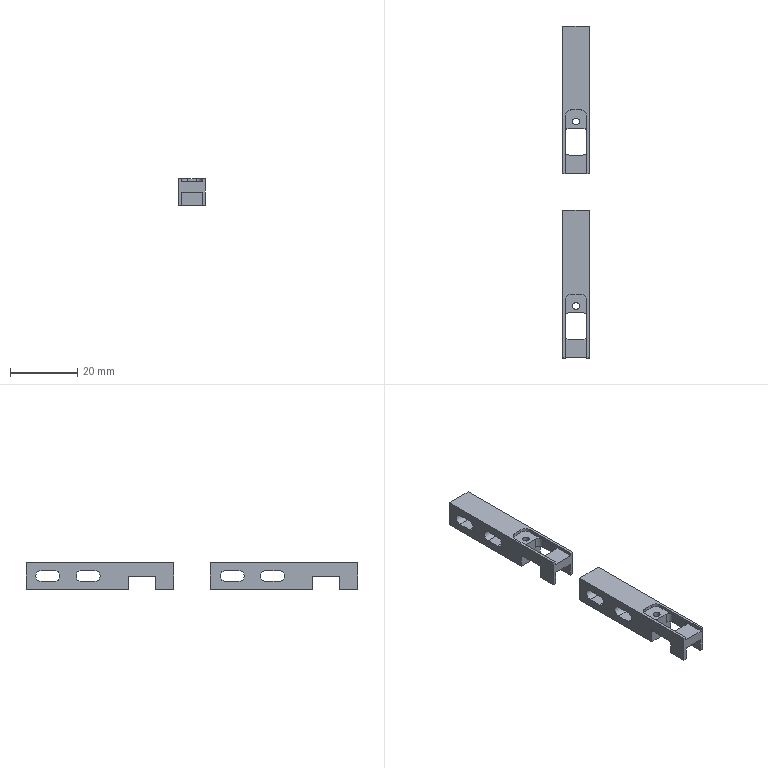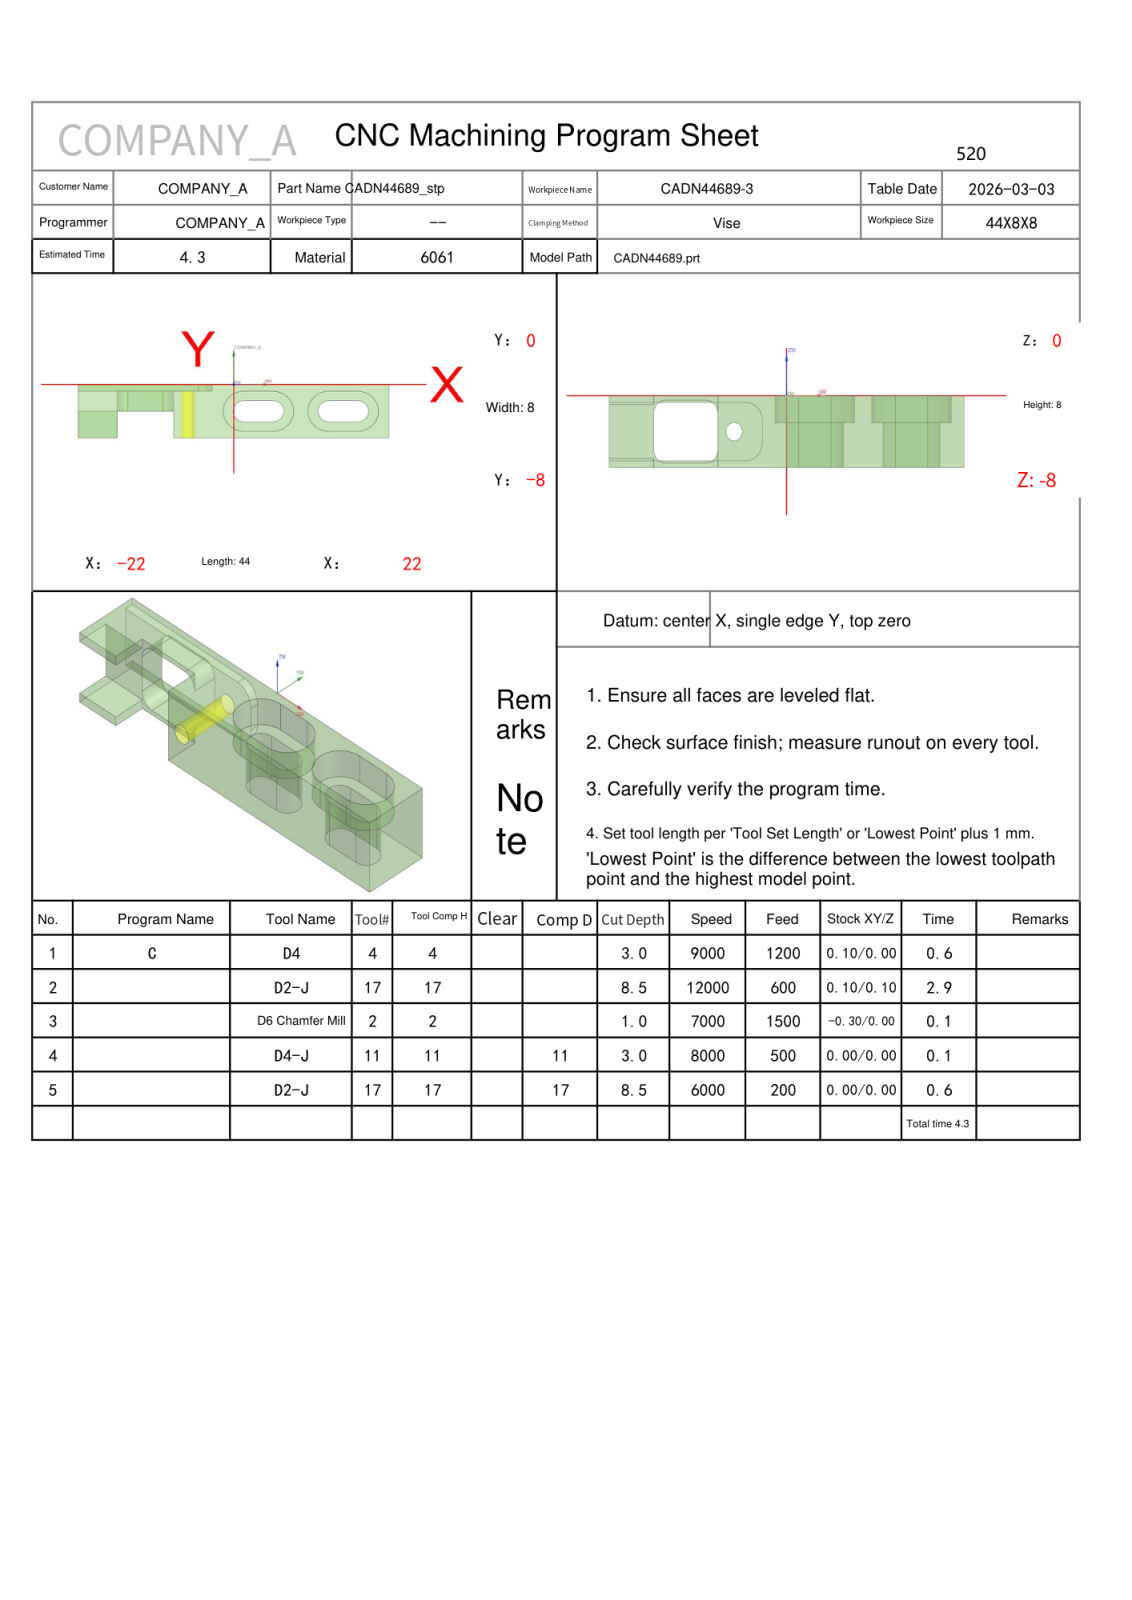NC program | NX | posted by the shop | part box 8 x 99 x 8 mm
Whole program, first 1224 of 1549 lines:
%
O0001
(Machine time: 5.15 MIN)
(===Total Tool:4===)
(T4=D4      D=4.   R=0.   D-  H04 Z=-3.   )
(T17=D2-J   D=2.   R=0.   D-  H17 Z=-8.5  )
(T2=D6 Chamfer Mill   D=6.   R=0.   D-  H02 Z=-1.   )
(T11=D4-J   D=4.   R=0.   D11 H11 Z=-3.   )
G80 G90 G17 G49 G40
G91 G28 Z0
M01
N1 T04 M06
(D4  D=4. R=0. H=04 ce=0.10 di=0.00)
G00 G90 G54 X3.5 Y-3.1 M03 S9000
G43 H04 Z50.
M08
Z.5
G01 X1.5 Z.479 F1200.
G03 X.6 Y-4. Z.464 I0.0 J-.9
X1.5 Y-4.9 Z.448 I.9 J0.0
G01 X5.5 Z.406
G03 X6.4 Y-4. Z.391 I0.0 J.9
X5.5 Y-3.1 Z.376 I-.9 J0.0
G01 X1.5 Z.333
G03 X.6 Y-4. Z.318 I0.0 J-.9
X1.5 Y-4.9 Z.303 I.9 J0.0
G01 X5.5 Z.26
G03 X6.4 Y-4. Z.245 I0.0 J.9
X5.5 Y-3.1 Z.23 I-.9 J0.0
G01 X1.5 Z.187
G03 X.6 Y-4. Z.172 I0.0 J-.9
X1.5 Y-4.9 Z.157 I.9 J0.0
G01 X5.5 Z.114
G03 X6.4 Y-4. Z.099 I0.0 J.9
X5.5 Y-3.1 Z.084 I-.9 J0.0
G01 X1.5 Z.041
G03 X.6 Y-4. Z.026 I0.0 J-.9
X1.5 Y-4.9 Z.011 I.9 J0.0
G01 X5.5 Z-.032
G03 X6.4 Y-4. Z-.047 I0.0 J.9
X5.5 Y-3.1 Z-.062 I-.9 J0.0
G01 X1.5 Z-.105
G03 X.6 Y-4. Z-.12 I0.0 J-.9
X1.5 Y-4.9 Z-.135 I.9 J0.0
G01 X5.5 Z-.178
G03 X6.4 Y-4. Z-.193 I0.0 J.9
X5.5 Y-3.1 Z-.208 I-.9 J0.0
G01 X1.5 Z-.251
G03 X.6 Y-4. Z-.266 I0.0 J-.9
X1.5 Y-4.9 Z-.281 I.9 J0.0
G01 X5.5 Z-.323
G03 X6.4 Y-4. Z-.339 I0.0 J.9
X5.5 Y-3.1 Z-.354 I-.9 J0.0
G01 X1.5 Z-.396
G03 X.6 Y-4. Z-.411 I0.0 J-.9
X1.5 Y-4.9 Z-.427 I.9 J0.0
G01 X5.5 Z-.469
G03 X6.4 Y-4. Z-.484 I0.0 J.9
X5.5 Y-3.1 Z-.499 I-.9 J0.0
G01 X1.5 Z-.542
G03 X.6 Y-4. Z-.557 I0.0 J-.9
X1.5 Y-4.9 Z-.572 I.9 J0.0
G01 X5.5 Z-.615
G03 X6.4 Y-4. Z-.63 I0.0 J.9
X5.5 Y-3.1 Z-.645 I-.9 J0.0
G01 X1.5 Z-.688
G03 X.6 Y-4. Z-.703 I0.0 J-.9
X1.5 Y-4.9 Z-.718 I.9 J0.0
G01 X5.5 Z-.761
G03 X6.4 Y-4. Z-.776 I0.0 J.9
X5.5 Y-3.1 Z-.791 I-.9 J0.0
G01 X1.5 Z-.834
G03 X.6 Y-4. Z-.849 I0.0 J-.9
X1.5 Y-4.9 Z-.864 I.9 J0.0
G01 X5.5 Z-.907
G03 X6.4 Y-4. Z-.922 I0.0 J.9
X5.5 Y-3.1 Z-.937 I-.9 J0.0
G01 X1.5 Z-.98
G03 X.6 Y-4. Z-.995 I0.0 J-.9
X1.5 Y-4.9 Z-1.01 I.9 J0.0
G01 X5.5 Z-1.053
G03 X6.4 Y-4. Z-1.068 I0.0 J.9
X5.5 Y-3.1 Z-1.083 I-.9 J0.0
G01 X1.5 Z-1.126
G03 X.6 Y-4. Z-1.141 I0.0 J-.9
X1.5 Y-4.9 Z-1.156 I.9 J0.0
G01 X5.5 Z-1.198
G03 X6.4 Y-4. Z-1.214 I0.0 J.9
X5.5 Y-3.1 Z-1.229 I-.9 J0.0
G01 X1.5 Z-1.271
G03 X.6 Y-4. Z-1.286 I0.0 J-.9
X1.5 Y-4.9 Z-1.302 I.9 J0.0
G01 X5.5 Z-1.344
G03 X6.4 Y-4. Z-1.359 I0.0 J.9
X5.5 Y-3.1 Z-1.374 I-.9 J0.0
G01 X1.5 Z-1.417
G03 X.6 Y-4. Z-1.432 I0.0 J-.9
X1.5 Y-4.9 Z-1.447 I.9 J0.0
G01 X5.5 Z-1.49
G03 X6.4 Y-4. Z-1.505 I0.0 J.9
X5.5 Y-3.1 Z-1.52 I-.9 J0.0
G01 X1.5 Z-1.563
G03 X.6 Y-4. Z-1.578 I0.0 J-.9
X1.5 Y-4.9 Z-1.593 I.9 J0.0
G01 X5.5 Z-1.636
G03 X6.4 Y-4. Z-1.651 I0.0 J.9
X5.5 Y-3.1 Z-1.666 I-.9 J0.0
G01 X1.5 Z-1.709
G03 X.6 Y-4. Z-1.724 I0.0 J-.9
X1.5 Y-4.9 Z-1.739 I.9 J0.0
G01 X5.5 Z-1.782
G03 X6.4 Y-4. Z-1.797 I0.0 J.9
X5.5 Y-3.1 Z-1.812 I-.9 J0.0
G01 X1.5 Z-1.855
G03 X.6 Y-4. Z-1.87 I0.0 J-.9
X1.5 Y-4.9 Z-1.885 I.9 J0.0
G01 X5.5 Z-1.928
G03 X6.4 Y-4. Z-1.943 I0.0 J.9
X5.5 Y-3.1 Z-1.958 I-.9 J0.0
G01 X1.5 Z-2.001
G03 X.6 Y-4. Z-2.016 I0.0 J-.9
X1.5 Y-4.9 Z-2.031 I.9 J0.0
G01 X5.5 Z-2.073
G03 X6.4 Y-4. Z-2.089 I0.0 J.9
X5.5 Y-3.1 Z-2.104 I-.9 J0.0
G01 X1.5 Z-2.146
G03 X.6 Y-4. Z-2.161 I0.0 J-.9
X1.5 Y-4.9 Z-2.177 I.9 J0.0
G01 X5.5 Z-2.219
G03 X6.4 Y-4. Z-2.234 I0.0 J.9
X5.5 Y-3.1 Z-2.249 I-.9 J0.0
G01 X1.5 Z-2.292
G03 X.6 Y-4. Z-2.307 I0.0 J-.9
X1.5 Y-4.9 Z-2.322 I.9 J0.0
G01 X5.5 Z-2.365
G03 X6.4 Y-4. Z-2.38 I0.0 J.9
X5.5 Y-3.1 Z-2.395 I-.9 J0.0
G01 X1.5 Z-2.438
G03 X.6 Y-4. Z-2.453 I0.0 J-.9
X1.5 Y-4.9 Z-2.468 I.9 J0.0
G01 X5.5 Z-2.511
G03 X6.4 Y-4. Z-2.526 I0.0 J.9
X5.5 Y-3.1 Z-2.541 I-.9 J0.0
G01 X1.5 Z-2.584
G03 X.6 Y-4. Z-2.599 I0.0 J-.9
X1.5 Y-4.9 Z-2.614 I.9 J0.0
G01 X5.5 Z-2.657
G03 X6.4 Y-4. Z-2.672 I0.0 J.9
X5.5 Y-3.1 Z-2.687 I-.9 J0.0
G01 X1.5 Z-2.73
G03 X.6 Y-4. Z-2.745 I0.0 J-.9
X1.5 Y-4.9 Z-2.76 I.9 J0.0
G01 X5.5 Z-2.803
G03 X6.4 Y-4. Z-2.818 I0.0 J.9
X5.5 Y-3.1 Z-2.833 I-.9 J0.0
G01 X1.5 Z-2.876
G03 X.6 Y-4. Z-2.891 I0.0 J-.9
X1.5 Y-4.9 Z-2.906 I.9 J0.0
G01 X5.5 Z-2.948
G03 X6.4 Y-4. Z-2.964 I0.0 J.9
X5.5 Y-3.1 Z-2.979 I-.9 J0.0
G01 X3.5 Z-3.
X1.5
G03 X.6 Y-4. I0.0 J-.9
X1.5 Y-4.9 I.9 J0.0
G01 X5.5
G03 X6.4 Y-4. I0.0 J.9
X5.5 Y-3.1 I-.9 J0.0
G01 X3.5
X3.
Z-2.
G00 Z50.
X15.5
Z.5
G01 X13.5 Z.479
G03 X12.6 Y-4. Z.464 I0.0 J-.9
X13.5 Y-4.9 Z.448 I.9 J0.0
G01 X17.5 Z.406
G03 X18.4 Y-4. Z.391 I0.0 J.9
X17.5 Y-3.1 Z.376 I-.9 J0.0
G01 X13.5 Z.333
G03 X12.6 Y-4. Z.318 I0.0 J-.9
X13.5 Y-4.9 Z.303 I.9 J0.0
G01 X17.5 Z.26
G03 X18.4 Y-4. Z.245 I0.0 J.9
X17.5 Y-3.1 Z.23 I-.9 J0.0
G01 X13.5 Z.187
G03 X12.6 Y-4. Z.172 I0.0 J-.9
X13.5 Y-4.9 Z.157 I.9 J0.0
G01 X17.5 Z.114
G03 X18.4 Y-4. Z.099 I0.0 J.9
X17.5 Y-3.1 Z.084 I-.9 J0.0
G01 X13.5 Z.041
G03 X12.6 Y-4. Z.026 I0.0 J-.9
X13.5 Y-4.9 Z.011 I.9 J0.0
G01 X17.5 Z-.032
G03 X18.4 Y-4. Z-.047 I0.0 J.9
X17.5 Y-3.1 Z-.062 I-.9 J0.0
G01 X13.5 Z-.105
G03 X12.6 Y-4. Z-.12 I0.0 J-.9
X13.5 Y-4.9 Z-.135 I.9 J0.0
G01 X17.5 Z-.178
G03 X18.4 Y-4. Z-.193 I0.0 J.9
X17.5 Y-3.1 Z-.208 I-.9 J0.0
G01 X13.5 Z-.251
G03 X12.6 Y-4. Z-.266 I0.0 J-.9
X13.5 Y-4.9 Z-.281 I.9 J0.0
G01 X17.5 Z-.323
G03 X18.4 Y-4. Z-.339 I0.0 J.9
X17.5 Y-3.1 Z-.354 I-.9 J0.0
G01 X13.5 Z-.396
G03 X12.6 Y-4. Z-.411 I0.0 J-.9
X13.5 Y-4.9 Z-.427 I.9 J0.0
G01 X17.5 Z-.469
G03 X18.4 Y-4. Z-.484 I0.0 J.9
X17.5 Y-3.1 Z-.499 I-.9 J0.0
G01 X13.5 Z-.542
G03 X12.6 Y-4. Z-.557 I0.0 J-.9
X13.5 Y-4.9 Z-.572 I.9 J0.0
G01 X17.5 Z-.615
G03 X18.4 Y-4. Z-.63 I0.0 J.9
X17.5 Y-3.1 Z-.645 I-.9 J0.0
G01 X13.5 Z-.688
G03 X12.6 Y-4. Z-.703 I0.0 J-.9
X13.5 Y-4.9 Z-.718 I.9 J0.0
G01 X17.5 Z-.761
G03 X18.4 Y-4. Z-.776 I0.0 J.9
X17.5 Y-3.1 Z-.791 I-.9 J0.0
G01 X13.5 Z-.834
G03 X12.6 Y-4. Z-.849 I0.0 J-.9
X13.5 Y-4.9 Z-.864 I.9 J0.0
G01 X17.5 Z-.907
G03 X18.4 Y-4. Z-.922 I0.0 J.9
X17.5 Y-3.1 Z-.937 I-.9 J0.0
G01 X13.5 Z-.98
G03 X12.6 Y-4. Z-.995 I0.0 J-.9
X13.5 Y-4.9 Z-1.01 I.9 J0.0
G01 X17.5 Z-1.053
G03 X18.4 Y-4. Z-1.068 I0.0 J.9
X17.5 Y-3.1 Z-1.083 I-.9 J0.0
G01 X13.5 Z-1.126
G03 X12.6 Y-4. Z-1.141 I0.0 J-.9
X13.5 Y-4.9 Z-1.156 I.9 J0.0
G01 X17.5 Z-1.198
G03 X18.4 Y-4. Z-1.214 I0.0 J.9
X17.5 Y-3.1 Z-1.229 I-.9 J0.0
G01 X13.5 Z-1.271
G03 X12.6 Y-4. Z-1.286 I0.0 J-.9
X13.5 Y-4.9 Z-1.302 I.9 J0.0
G01 X17.5 Z-1.344
G03 X18.4 Y-4. Z-1.359 I0.0 J.9
X17.5 Y-3.1 Z-1.374 I-.9 J0.0
G01 X13.5 Z-1.417
G03 X12.6 Y-4. Z-1.432 I0.0 J-.9
X13.5 Y-4.9 Z-1.447 I.9 J0.0
G01 X17.5 Z-1.49
G03 X18.4 Y-4. Z-1.505 I0.0 J.9
X17.5 Y-3.1 Z-1.52 I-.9 J0.0
G01 X13.5 Z-1.563
G03 X12.6 Y-4. Z-1.578 I0.0 J-.9
X13.5 Y-4.9 Z-1.593 I.9 J0.0
G01 X17.5 Z-1.636
G03 X18.4 Y-4. Z-1.651 I0.0 J.9
X17.5 Y-3.1 Z-1.666 I-.9 J0.0
G01 X13.5 Z-1.709
G03 X12.6 Y-4. Z-1.724 I0.0 J-.9
X13.5 Y-4.9 Z-1.739 I.9 J0.0
G01 X17.5 Z-1.782
G03 X18.4 Y-4. Z-1.797 I0.0 J.9
X17.5 Y-3.1 Z-1.812 I-.9 J0.0
G01 X13.5 Z-1.855
G03 X12.6 Y-4. Z-1.87 I0.0 J-.9
X13.5 Y-4.9 Z-1.885 I.9 J0.0
G01 X17.5 Z-1.928
G03 X18.4 Y-4. Z-1.943 I0.0 J.9
X17.5 Y-3.1 Z-1.958 I-.9 J0.0
G01 X13.5 Z-2.001
G03 X12.6 Y-4. Z-2.016 I0.0 J-.9
X13.5 Y-4.9 Z-2.031 I.9 J0.0
G01 X17.5 Z-2.073
G03 X18.4 Y-4. Z-2.089 I0.0 J.9
X17.5 Y-3.1 Z-2.104 I-.9 J0.0
G01 X13.5 Z-2.146
G03 X12.6 Y-4. Z-2.161 I0.0 J-.9
X13.5 Y-4.9 Z-2.177 I.9 J0.0
G01 X17.5 Z-2.219
G03 X18.4 Y-4. Z-2.234 I0.0 J.9
X17.5 Y-3.1 Z-2.249 I-.9 J0.0
G01 X13.5 Z-2.292
G03 X12.6 Y-4. Z-2.307 I0.0 J-.9
X13.5 Y-4.9 Z-2.322 I.9 J0.0
G01 X17.5 Z-2.365
G03 X18.4 Y-4. Z-2.38 I0.0 J.9
X17.5 Y-3.1 Z-2.395 I-.9 J0.0
G01 X13.5 Z-2.438
G03 X12.6 Y-4. Z-2.453 I0.0 J-.9
X13.5 Y-4.9 Z-2.468 I.9 J0.0
G01 X17.5 Z-2.511
G03 X18.4 Y-4. Z-2.526 I0.0 J.9
X17.5 Y-3.1 Z-2.541 I-.9 J0.0
G01 X13.5 Z-2.584
G03 X12.6 Y-4. Z-2.599 I0.0 J-.9
X13.5 Y-4.9 Z-2.614 I.9 J0.0
G01 X17.5 Z-2.657
G03 X18.4 Y-4. Z-2.672 I0.0 J.9
X17.5 Y-3.1 Z-2.687 I-.9 J0.0
G01 X13.5 Z-2.73
G03 X12.6 Y-4. Z-2.745 I0.0 J-.9
X13.5 Y-4.9 Z-2.76 I.9 J0.0
G01 X17.5 Z-2.803
G03 X18.4 Y-4. Z-2.818 I0.0 J.9
X17.5 Y-3.1 Z-2.833 I-.9 J0.0
G01 X13.5 Z-2.876
G03 X12.6 Y-4. Z-2.891 I0.0 J-.9
X13.5 Y-4.9 Z-2.906 I.9 J0.0
G01 X17.5 Z-2.948
G03 X18.4 Y-4. Z-2.964 I0.0 J.9
X17.5 Y-3.1 Z-2.979 I-.9 J0.0
G01 X15.5 Z-3.
X13.5
G03 X12.6 Y-4. I0.0 J-.9
X13.5 Y-4.9 I.9 J0.0
G01 X17.5
G03 X18.4 Y-4. I0.0 J.9
X17.5 Y-3.1 I-.9 J0.0
G01 X15.5
X15.
Z-2.
G00 Z50.
G91 G28 Z0.0
M05
M09
G91 G28 Z0.0
M01
N2 T17 M06
(D2-J  D=2. R=0. H=17 ce=0.10 di=0.10)
G00 G90 G54 X15.5 Y-3.5 M03 S12000
G43 H17 Z50.
M08
Z-2.5
G01 X13.5 Z-2.514 F600.
G03 X13. Y-4. Z-2.52 I0.0 J-.5
X13.5 Y-4.5 Z-2.526 I.5 J0.0
G01 X17.5 Z-2.554
G03 X18. Y-4. Z-2.56 I0.0 J.5
X17.5 Y-3.5 Z-2.566 I-.5 J0.0
G01 X13.5 Z-2.594
G03 X13. Y-4. Z-2.6 I0.0 J-.5
X13.5 Y-4.5 Z-2.606 I.5 J0.0
G01 X17.5 Z-2.634
G03 X18. Y-4. Z-2.64 I0.0 J.5
X17.5 Y-3.5 Z-2.646 I-.5 J0.0
G01 X13.5 Z-2.674
G03 X13. Y-4. Z-2.68 I0.0 J-.5
X13.5 Y-4.5 Z-2.686 I.5 J0.0
G01 X17.5 Z-2.714
G03 X18. Y-4. Z-2.72 I0.0 J.5
X17.5 Y-3.5 Z-2.726 I-.5 J0.0
G01 X13.5 Z-2.754
G03 X13. Y-4. Z-2.76 I0.0 J-.5
X13.5 Y-4.5 Z-2.766 I.5 J0.0
G01 X17.5 Z-2.794
G03 X18. Y-4. Z-2.8 I0.0 J.5
X17.5 Y-3.5 Z-2.806 I-.5 J0.0
G01 X13.5 Z-2.834
G03 X13. Y-4. Z-2.84 I0.0 J-.5
X13.5 Y-4.5 Z-2.846 I.5 J0.0
G01 X17.5 Z-2.874
G03 X18. Y-4. Z-2.88 I0.0 J.5
X17.5 Y-3.5 Z-2.886 I-.5 J0.0
G01 X13.5 Z-2.914
G03 X13. Y-4. Z-2.92 I0.0 J-.5
X13.5 Y-4.5 Z-2.926 I.5 J0.0
G01 X17.5 Z-2.954
G03 X18. Y-4. Z-2.96 I0.0 J.5
X17.5 Y-3.5 Z-2.966 I-.5 J0.0
G01 X13.5 Z-2.994
G03 X13. Y-4. Z-3. I0.0 J-.5
X13.5 Y-4.5 Z-3.006 I.5 J0.0
G01 X17.5 Z-3.034
G03 X18. Y-4. Z-3.04 I0.0 J.5
X17.5 Y-3.5 Z-3.046 I-.5 J0.0
G01 X13.5 Z-3.074
G03 X13. Y-4. Z-3.08 I0.0 J-.5
X13.5 Y-4.5 Z-3.086 I.5 J0.0
G01 X17.5 Z-3.114
G03 X18. Y-4. Z-3.12 I0.0 J.5
X17.5 Y-3.5 Z-3.126 I-.5 J0.0
G01 X13.5 Z-3.154
G03 X13. Y-4. Z-3.16 I0.0 J-.5
X13.5 Y-4.5 Z-3.166 I.5 J0.0
G01 X17.5 Z-3.194
G03 X18. Y-4. Z-3.2 I0.0 J.5
X17.5 Y-3.5 Z-3.206 I-.5 J0.0
G01 X13.5 Z-3.234
G03 X13. Y-4. Z-3.24 I0.0 J-.5
X13.5 Y-4.5 Z-3.246 I.5 J0.0
G01 X17.5 Z-3.274
G03 X18. Y-4. Z-3.28 I0.0 J.5
X17.5 Y-3.5 Z-3.286 I-.5 J0.0
G01 X13.5 Z-3.314
G03 X13. Y-4. Z-3.32 I0.0 J-.5
X13.5 Y-4.5 Z-3.326 I.5 J0.0
G01 X17.5 Z-3.354
G03 X18. Y-4. Z-3.36 I0.0 J.5
X17.5 Y-3.5 Z-3.366 I-.5 J0.0
G01 X13.5 Z-3.394
G03 X13. Y-4. Z-3.4 I0.0 J-.5
X13.5 Y-4.5 Z-3.406 I.5 J0.0
G01 X17.5 Z-3.434
G03 X18. Y-4. Z-3.44 I0.0 J.5
X17.5 Y-3.5 Z-3.446 I-.5 J0.0
G01 X13.5 Z-3.474
G03 X13. Y-4. Z-3.48 I0.0 J-.5
X13.5 Y-4.5 Z-3.486 I.5 J0.0
G01 X17.5 Z-3.514
G03 X18. Y-4. Z-3.52 I0.0 J.5
X17.5 Y-3.5 Z-3.526 I-.5 J0.0
G01 X13.5 Z-3.554
G03 X13. Y-4. Z-3.56 I0.0 J-.5
X13.5 Y-4.5 Z-3.566 I.5 J0.0
G01 X17.5 Z-3.594
G03 X18. Y-4. Z-3.6 I0.0 J.5
X17.5 Y-3.5 Z-3.606 I-.5 J0.0
G01 X13.5 Z-3.634
G03 X13. Y-4. Z-3.64 I0.0 J-.5
X13.5 Y-4.5 Z-3.646 I.5 J0.0
G01 X17.5 Z-3.674
G03 X18. Y-4. Z-3.68 I0.0 J.5
X17.5 Y-3.5 Z-3.686 I-.5 J0.0
G01 X13.5 Z-3.714
G03 X13. Y-4. Z-3.72 I0.0 J-.5
X13.5 Y-4.5 Z-3.726 I.5 J0.0
G01 X17.5 Z-3.754
G03 X18. Y-4. Z-3.76 I0.0 J.5
X17.5 Y-3.5 Z-3.766 I-.5 J0.0
G01 X13.5 Z-3.794
G03 X13. Y-4. Z-3.8 I0.0 J-.5
X13.5 Y-4.5 Z-3.806 I.5 J0.0
G01 X17.5 Z-3.834
G03 X18. Y-4. Z-3.84 I0.0 J.5
X17.5 Y-3.5 Z-3.846 I-.5 J0.0
G01 X13.5 Z-3.874
G03 X13. Y-4. Z-3.88 I0.0 J-.5
X13.5 Y-4.5 Z-3.886 I.5 J0.0
G01 X17.5 Z-3.914
G03 X18. Y-4. Z-3.92 I0.0 J.5
X17.5 Y-3.5 Z-3.926 I-.5 J0.0
G01 X13.5 Z-3.954
G03 X13. Y-4. Z-3.96 I0.0 J-.5
X13.5 Y-4.5 Z-3.966 I.5 J0.0
G01 X17.5 Z-3.994
G03 X18. Y-4. Z-4. I0.0 J.5
X17.5 Y-3.5 Z-4.006 I-.5 J0.0
G01 X13.5 Z-4.034
G03 X13. Y-4. Z-4.04 I0.0 J-.5
X13.5 Y-4.5 Z-4.046 I.5 J0.0
G01 X17.5 Z-4.074
G03 X18. Y-4. Z-4.08 I0.0 J.5
X17.5 Y-3.5 Z-4.086 I-.5 J0.0
G01 X13.5 Z-4.114
G03 X13. Y-4. Z-4.12 I0.0 J-.5
X13.5 Y-4.5 Z-4.126 I.5 J0.0
G01 X17.5 Z-4.154
G03 X18. Y-4. Z-4.16 I0.0 J.5
X17.5 Y-3.5 Z-4.166 I-.5 J0.0
G01 X13.5 Z-4.194
G03 X13. Y-4. Z-4.2 I0.0 J-.5
X13.5 Y-4.5 Z-4.206 I.5 J0.0
G01 X17.5 Z-4.234
G03 X18. Y-4. Z-4.24 I0.0 J.5
X17.5 Y-3.5 Z-4.246 I-.5 J0.0
G01 X13.5 Z-4.274
G03 X13. Y-4. Z-4.28 I0.0 J-.5
X13.5 Y-4.5 Z-4.286 I.5 J0.0
G01 X17.5 Z-4.314
G03 X18. Y-4. Z-4.32 I0.0 J.5
X17.5 Y-3.5 Z-4.326 I-.5 J0.0
G01 X13.5 Z-4.354
G03 X13. Y-4. Z-4.36 I0.0 J-.5
X13.5 Y-4.5 Z-4.366 I.5 J0.0
G01 X17.5 Z-4.394
G03 X18. Y-4. Z-4.4 I0.0 J.5
X17.5 Y-3.5 Z-4.406 I-.5 J0.0
G01 X13.5 Z-4.434
G03 X13. Y-4. Z-4.44 I0.0 J-.5
X13.5 Y-4.5 Z-4.446 I.5 J0.0
G01 X17.5 Z-4.474
G03 X18. Y-4. Z-4.48 I0.0 J.5
X17.5 Y-3.5 Z-4.486 I-.5 J0.0
G01 X13.5 Z-4.514
G03 X13. Y-4. Z-4.52 I0.0 J-.5
X13.5 Y-4.5 Z-4.526 I.5 J0.0
G01 X17.5 Z-4.554
G03 X18. Y-4. Z-4.56 I0.0 J.5
X17.5 Y-3.5 Z-4.566 I-.5 J0.0
G01 X13.5 Z-4.594
G03 X13. Y-4. Z-4.6 I0.0 J-.5
X13.5 Y-4.5 Z-4.606 I.5 J0.0
G01 X17.5 Z-4.634
G03 X18. Y-4. Z-4.64 I0.0 J.5
X17.5 Y-3.5 Z-4.646 I-.5 J0.0
G01 X13.5 Z-4.674
G03 X13. Y-4. Z-4.68 I0.0 J-.5
X13.5 Y-4.5 Z-4.686 I.5 J0.0
G01 X17.5 Z-4.714
G03 X18. Y-4. Z-4.72 I0.0 J.5
X17.5 Y-3.5 Z-4.726 I-.5 J0.0
G01 X13.5 Z-4.754
G03 X13. Y-4. Z-4.76 I0.0 J-.5
X13.5 Y-4.5 Z-4.766 I.5 J0.0
G01 X17.5 Z-4.794
G03 X18. Y-4. Z-4.8 I0.0 J.5
X17.5 Y-3.5 Z-4.806 I-.5 J0.0
G01 X13.5 Z-4.834
G03 X13. Y-4. Z-4.84 I0.0 J-.5
X13.5 Y-4.5 Z-4.846 I.5 J0.0
G01 X17.5 Z-4.874
G03 X18. Y-4. Z-4.88 I0.0 J.5
X17.5 Y-3.5 Z-4.886 I-.5 J0.0
G01 X13.5 Z-4.914
G03 X13. Y-4. Z-4.92 I0.0 J-.5
X13.5 Y-4.5 Z-4.926 I.5 J0.0
G01 X17.5 Z-4.954
G03 X18. Y-4. Z-4.96 I0.0 J.5
X17.5 Y-3.5 Z-4.966 I-.5 J0.0
G01 X13.5 Z-4.994
G03 X13. Y-4. Z-5. I0.0 J-.5
X13.5 Y-4.5 Z-5.006 I.5 J0.0
G01 X17.5 Z-5.034
G03 X18. Y-4. Z-5.04 I0.0 J.5
X17.5 Y-3.5 Z-5.046 I-.5 J0.0
G01 X13.5 Z-5.074
G03 X13. Y-4. Z-5.08 I0.0 J-.5
X13.5 Y-4.5 Z-5.086 I.5 J0.0
G01 X17.5 Z-5.114
G03 X18. Y-4. Z-5.12 I0.0 J.5
X17.5 Y-3.5 Z-5.126 I-.5 J0.0
G01 X13.5 Z-5.154
G03 X13. Y-4. Z-5.16 I0.0 J-.5
X13.5 Y-4.5 Z-5.166 I.5 J0.0
G01 X17.5 Z-5.194
G03 X18. Y-4. Z-5.2 I0.0 J.5
X17.5 Y-3.5 Z-5.206 I-.5 J0.0
G01 X13.5 Z-5.234
G03 X13. Y-4. Z-5.24 I0.0 J-.5
X13.5 Y-4.5 Z-5.246 I.5 J0.0
G01 X17.5 Z-5.274
G03 X18. Y-4. Z-5.28 I0.0 J.5
X17.5 Y-3.5 Z-5.286 I-.5 J0.0
G01 X13.5 Z-5.314
G03 X13. Y-4. Z-5.32 I0.0 J-.5
X13.5 Y-4.5 Z-5.326 I.5 J0.0
G01 X17.5 Z-5.354
G03 X18. Y-4. Z-5.36 I0.0 J.5
X17.5 Y-3.5 Z-5.366 I-.5 J0.0
G01 X13.5 Z-5.394
G03 X13. Y-4. Z-5.4 I0.0 J-.5
X13.5 Y-4.5 Z-5.406 I.5 J0.0
G01 X17.5 Z-5.434
G03 X18. Y-4. Z-5.44 I0.0 J.5
X17.5 Y-3.5 Z-5.446 I-.5 J0.0
G01 X13.5 Z-5.474
G03 X13. Y-4. Z-5.48 I0.0 J-.5
X13.5 Y-4.5 Z-5.486 I.5 J0.0
G01 X17.5 Z-5.514
G03 X18. Y-4. Z-5.52 I0.0 J.5
X17.5 Y-3.5 Z-5.526 I-.5 J0.0
G01 X13.5 Z-5.554
G03 X13. Y-4. Z-5.56 I0.0 J-.5
X13.5 Y-4.5 Z-5.566 I.5 J0.0
G01 X17.5 Z-5.594
G03 X18. Y-4. Z-5.6 I0.0 J.5
X17.5 Y-3.5 Z-5.606 I-.5 J0.0
G01 X13.5 Z-5.634
G03 X13. Y-4. Z-5.64 I0.0 J-.5
X13.5 Y-4.5 Z-5.646 I.5 J0.0
G01 X17.5 Z-5.674
G03 X18. Y-4. Z-5.68 I0.0 J.5
X17.5 Y-3.5 Z-5.686 I-.5 J0.0
G01 X13.5 Z-5.714
G03 X13. Y-4. Z-5.72 I0.0 J-.5
X13.5 Y-4.5 Z-5.726 I.5 J0.0
G01 X17.5 Z-5.754
G03 X18. Y-4. Z-5.76 I0.0 J.5
X17.5 Y-3.5 Z-5.766 I-.5 J0.0
G01 X13.5 Z-5.794
G03 X13. Y-4. Z-5.8 I0.0 J-.5
X13.5 Y-4.5 Z-5.806 I.5 J0.0
G01 X17.5 Z-5.834
G03 X18. Y-4. Z-5.84 I0.0 J.5
X17.5 Y-3.5 Z-5.846 I-.5 J0.0
G01 X13.5 Z-5.874
G03 X13. Y-4. Z-5.88 I0.0 J-.5
X13.5 Y-4.5 Z-5.886 I.5 J0.0
G01 X17.5 Z-5.914
G03 X18. Y-4. Z-5.92 I0.0 J.5
X17.5 Y-3.5 Z-5.926 I-.5 J0.0
G01 X13.5 Z-5.954
G03 X13. Y-4. Z-5.96 I0.0 J-.5
X13.5 Y-4.5 Z-5.966 I.5 J0.0
G01 X17.5 Z-5.994
G03 X18. Y-4. Z-6. I0.0 J.5
X17.5 Y-3.5 Z-6.006 I-.5 J0.0
G01 X13.5 Z-6.034
G03 X13. Y-4. Z-6.04 I0.0 J-.5
X13.5 Y-4.5 Z-6.046 I.5 J0.0
G01 X17.5 Z-6.074
G03 X18. Y-4. Z-6.08 I0.0 J.5
X17.5 Y-3.5 Z-6.086 I-.5 J0.0
G01 X13.5 Z-6.114
G03 X13. Y-4. Z-6.12 I0.0 J-.5
X13.5 Y-4.5 Z-6.126 I.5 J0.0
G01 X17.5 Z-6.154
G03 X18. Y-4. Z-6.16 I0.0 J.5
X17.5 Y-3.5 Z-6.166 I-.5 J0.0
G01 X13.5 Z-6.194
G03 X13. Y-4. Z-6.2 I0.0 J-.5
X13.5 Y-4.5 Z-6.206 I.5 J0.0
G01 X17.5 Z-6.234
G03 X18. Y-4. Z-6.24 I0.0 J.5
X17.5 Y-3.5 Z-6.246 I-.5 J0.0
G01 X13.5 Z-6.274
G03 X13. Y-4. Z-6.28 I0.0 J-.5
X13.5 Y-4.5 Z-6.286 I.5 J0.0
G01 X17.5 Z-6.314
G03 X18. Y-4. Z-6.32 I0.0 J.5
X17.5 Y-3.5 Z-6.326 I-.5 J0.0
G01 X13.5 Z-6.354
G03 X13. Y-4. Z-6.36 I0.0 J-.5
X13.5 Y-4.5 Z-6.366 I.5 J0.0
G01 X17.5 Z-6.394
G03 X18. Y-4. Z-6.4 I0.0 J.5
X17.5 Y-3.5 Z-6.406 I-.5 J0.0
G01 X13.5 Z-6.434
G03 X13. Y-4. Z-6.44 I0.0 J-.5
X13.5 Y-4.5 Z-6.446 I.5 J0.0
G01 X17.5 Z-6.474
G03 X18. Y-4. Z-6.48 I0.0 J.5
X17.5 Y-3.5 Z-6.486 I-.5 J0.0
G01 X13.5 Z-6.514
G03 X13. Y-4. Z-6.52 I0.0 J-.5
X13.5 Y-4.5 Z-6.526 I.5 J0.0
G01 X17.5 Z-6.554
G03 X18. Y-4. Z-6.56 I0.0 J.5
X17.5 Y-3.5 Z-6.566 I-.5 J0.0
G01 X13.5 Z-6.594
G03 X13. Y-4. Z-6.6 I0.0 J-.5
X13.5 Y-4.5 Z-6.606 I.5 J0.0
G01 X17.5 Z-6.634
G03 X18. Y-4. Z-6.64 I0.0 J.5
X17.5 Y-3.5 Z-6.646 I-.5 J0.0
G01 X13.5 Z-6.674
G03 X13. Y-4. Z-6.68 I0.0 J-.5
X13.5 Y-4.5 Z-6.686 I.5 J0.0
G01 X17.5 Z-6.714
G03 X18. Y-4. Z-6.72 I0.0 J.5
X17.5 Y-3.5 Z-6.726 I-.5 J0.0
G01 X13.5 Z-6.754
G03 X13. Y-4. Z-6.76 I0.0 J-.5
X13.5 Y-4.5 Z-6.766 I.5 J0.0
G01 X17.5 Z-6.794
G03 X18. Y-4. Z-6.8 I0.0 J.5
X17.5 Y-3.5 Z-6.806 I-.5 J0.0
G01 X13.5 Z-6.834
G03 X13. Y-4. Z-6.84 I0.0 J-.5
X13.5 Y-4.5 Z-6.846 I.5 J0.0
G01 X17.5 Z-6.874
G03 X18. Y-4. Z-6.88 I0.0 J.5
X17.5 Y-3.5 Z-6.886 I-.5 J0.0
G01 X13.5 Z-6.914
G03 X13. Y-4. Z-6.92 I0.0 J-.5
X13.5 Y-4.5 Z-6.926 I.5 J0.0
G01 X17.5 Z-6.954
G03 X18. Y-4. Z-6.96 I0.0 J.5
X17.5 Y-3.5 Z-6.966 I-.5 J0.0
G01 X13.5 Z-6.994
G03 X13. Y-4. Z-7. I0.0 J-.5
X13.5 Y-4.5 Z-7.006 I.5 J0.0
G01 X17.5 Z-7.034
G03 X18. Y-4. Z-7.04 I0.0 J.5
X17.5 Y-3.5 Z-7.046 I-.5 J0.0
G01 X13.5 Z-7.074
G03 X13. Y-4. Z-7.08 I0.0 J-.5
X13.5 Y-4.5 Z-7.086 I.5 J0.0
G01 X17.5 Z-7.114
G03 X18. Y-4. Z-7.12 I0.0 J.5
X17.5 Y-3.5 Z-7.126 I-.5 J0.0
G01 X13.5 Z-7.154
G03 X13. Y-4. Z-7.16 I0.0 J-.5
X13.5 Y-4.5 Z-7.166 I.5 J0.0
G01 X17.5 Z-7.194
G03 X18. Y-4. Z-7.2 I0.0 J.5
X17.5 Y-3.5 Z-7.206 I-.5 J0.0
G01 X13.5 Z-7.234
G03 X13. Y-4. Z-7.24 I0.0 J-.5
X13.5 Y-4.5 Z-7.246 I.5 J0.0
G01 X17.5 Z-7.274
G03 X18. Y-4. Z-7.28 I0.0 J.5
X17.5 Y-3.5 Z-7.286 I-.5 J0.0
G01 X13.5 Z-7.314
G03 X13. Y-4. Z-7.32 I0.0 J-.5
X13.5 Y-4.5 Z-7.326 I.5 J0.0
G01 X17.5 Z-7.354
G03 X18. Y-4. Z-7.36 I0.0 J.5
X17.5 Y-3.5 Z-7.366 I-.5 J0.0
G01 X13.5 Z-7.394
G03 X13. Y-4. Z-7.4 I0.0 J-.5
X13.5 Y-4.5 Z-7.406 I.5 J0.0
G01 X17.5 Z-7.434
G03 X18. Y-4. Z-7.44 I0.0 J.5
X17.5 Y-3.5 Z-7.446 I-.5 J0.0
G01 X13.5 Z-7.474
G03 X13. Y-4. Z-7.48 I0.0 J-.5
X13.5 Y-4.5 Z-7.486 I.5 J0.0
G01 X17.5 Z-7.514
G03 X18. Y-4. Z-7.52 I0.0 J.5
X17.5 Y-3.5 Z-7.526 I-.5 J0.0
G01 X13.5 Z-7.554
G03 X13. Y-4. Z-7.56 I0.0 J-.5
X13.5 Y-4.5 Z-7.566 I.5 J0.0
G01 X17.5 Z-7.594
G03 X18. Y-4. Z-7.6 I0.0 J.5
X17.5 Y-3.5 Z-7.606 I-.5 J0.0
G01 X13.5 Z-7.634
G03 X13. Y-4. Z-7.64 I0.0 J-.5
X13.5 Y-4.5 Z-7.646 I.5 J0.0
G01 X17.5 Z-7.674
G03 X18. Y-4. Z-7.68 I0.0 J.5
X17.5 Y-3.5 Z-7.686 I-.5 J0.0
G01 X13.5 Z-7.714
G03 X13. Y-4. Z-7.72 I0.0 J-.5
X13.5 Y-4.5 Z-7.726 I.5 J0.0
G01 X17.5 Z-7.754
G03 X18. Y-4. Z-7.76 I0.0 J.5
X17.5 Y-3.5 Z-7.766 I-.5 J0.0
G01 X13.5 Z-7.794
G03 X13. Y-4. Z-7.8 I0.0 J-.5
X13.5 Y-4.5 Z-7.806 I.5 J0.0
G01 X17.5 Z-7.834
G03 X18. Y-4. Z-7.84 I0.0 J.5
X17.5 Y-3.5 Z-7.846 I-.5 J0.0
G01 X13.5 Z-7.874
G03 X13. Y-4. Z-7.88 I0.0 J-.5
X13.5 Y-4.5 Z-7.886 I.5 J0.0
G01 X17.5 Z-7.914
G03 X18. Y-4. Z-7.92 I0.0 J.5
X17.5 Y-3.5 Z-7.926 I-.5 J0.0
G01 X13.5 Z-7.954
G03 X13. Y-4. Z-7.96 I0.0 J-.5
X13.5 Y-4.5 Z-7.966 I.5 J0.0
G01 X17.5 Z-7.994
G03 X18. Y-4. Z-8. I0.0 J.5
X17.5 Y-3.5 Z-8.006 I-.5 J0.0
G01 X13.5 Z-8.034
G03 X13. Y-4. Z-8.04 I0.0 J-.5
X13.5 Y-4.5 Z-8.046 I.5 J0.0
G01 X17.5 Z-8.074
G03 X18. Y-4. Z-8.08 I0.0 J.5
X17.5 Y-3.5 Z-8.086 I-.5 J0.0
G01 X13.5 Z-8.114
G03 X13. Y-4. Z-8.12 I0.0 J-.5
X13.5 Y-4.5 Z-8.126 I.5 J0.0
G01 X17.5 Z-8.154
G03 X18. Y-4. Z-8.16 I0.0 J.5
X17.5 Y-3.5 Z-8.166 I-.5 J0.0
G01 X13.5 Z-8.194
G03 X13. Y-4. Z-8.2 I0.0 J-.5
X13.5 Y-4.5 Z-8.206 I.5 J0.0
G01 X17.5 Z-8.234
G03 X18. Y-4. Z-8.24 I0.0 J.5
X17.5 Y-3.5 Z-8.246 I-.5 J0.0
G01 X13.5 Z-8.274
G03 X13. Y-4. Z-8.28 I0.0 J-.5
X13.5 Y-4.5 Z-8.286 I.5 J0.0
G01 X17.5 Z-8.314
G03 X18. Y-4. Z-8.32 I0.0 J.5
X17.5 Y-3.5 Z-8.326 I-.5 J0.0
G01 X13.5 Z-8.354
G03 X13. Y-4. Z-8.36 I0.0 J-.5
X13.5 Y-4.5 Z-8.366 I.5 J0.0
G01 X17.5 Z-8.394
G03 X18. Y-4. Z-8.4 I0.0 J.5
X17.5 Y-3.5 Z-8.406 I-.5 J0.0
G01 X13.5 Z-8.434
G03 X13. Y-4. Z-8.44 I0.0 J-.5
X13.5 Y-4.5 Z-8.446 I.5 J0.0
G01 X17.5 Z-8.474
G03 X18. Y-4. Z-8.48 I0.0 J.5
X17.5 Y-3.5 Z-8.486 I-.5 J0.0
G01 X15.5 Z-8.5
X13.5
G03 X13. Y-4. I0.0 J-.5
X13.5 Y-4.5 I.5 J0.0
G01 X17.5
G03 X18. Y-4. I0.0 J.5
X17.5 Y-3.5 I-.5 J0.0
G01 X15.5
X15.
Z-7.5
G00 Z50.
X3.5
Z-2.5
G01 X1.5 Z-2.514
G03 X1. Y-4. Z-2.52 I0.0 J-.5
X1.5 Y-4.5 Z-2.526 I.5 J0.0
G01 X5.5 Z-2.554
G03 X6. Y-4. Z-2.56 I0.0 J.5
X5.5 Y-3.5 Z-2.566 I-.5 J0.0
G01 X1.5 Z-2.594
G03 X1. Y-4. Z-2.6 I0.0 J-.5
X1.5 Y-4.5 Z-2.606 I.5 J0.0
G01 X5.5 Z-2.634
G03 X6. Y-4. Z-2.64 I0.0 J.5
X5.5 Y-3.5 Z-2.646 I-.5 J0.0
G01 X1.5 Z-2.674
G03 X1. Y-4. Z-2.68 I0.0 J-.5
X1.5 Y-4.5 Z-2.686 I.5 J0.0
G01 X5.5 Z-2.714
G03 X6. Y-4. Z-2.72 I0.0 J.5
X5.5 Y-3.5 Z-2.726 I-.5 J0.0
G01 X1.5 Z-2.754
G03 X1. Y-4. Z-2.76 I0.0 J-.5
X1.5 Y-4.5 Z-2.766 I.5 J0.0
G01 X5.5 Z-2.794
G03 X6. Y-4. Z-2.8 I0.0 J.5
X5.5 Y-3.5 Z-2.806 I-.5 J0.0
G01 X1.5 Z-2.834
G03 X1. Y-4. Z-2.84 I0.0 J-.5
X1.5 Y-4.5 Z-2.846 I.5 J0.0
G01 X5.5 Z-2.874
G03 X6. Y-4. Z-2.88 I0.0 J.5
X5.5 Y-3.5 Z-2.886 I-.5 J0.0
G01 X1.5 Z-2.914
G03 X1. Y-4. Z-2.92 I0.0 J-.5
X1.5 Y-4.5 Z-2.926 I.5 J0.0
G01 X5.5 Z-2.954
G03 X6. Y-4. Z-2.96 I0.0 J.5
X5.5 Y-3.5 Z-2.966 I-.5 J0.0
G01 X1.5 Z-2.994
G03 X1. Y-4. Z-3. I0.0 J-.5
X1.5 Y-4.5 Z-3.006 I.5 J0.0
G01 X5.5 Z-3.034
G03 X6. Y-4. Z-3.04 I0.0 J.5
X5.5 Y-3.5 Z-3.046 I-.5 J0.0
G01 X1.5 Z-3.074
G03 X1. Y-4. Z-3.08 I0.0 J-.5
X1.5 Y-4.5 Z-3.086 I.5 J0.0
G01 X5.5 Z-3.114
G03 X6. Y-4. Z-3.12 I0.0 J.5
X5.5 Y-3.5 Z-3.126 I-.5 J0.0
G01 X1.5 Z-3.154
G03 X1. Y-4. Z-3.16 I0.0 J-.5
X1.5 Y-4.5 Z-3.166 I.5 J0.0
G01 X5.5 Z-3.194
G03 X6. Y-4. Z-3.2 I0.0 J.5
X5.5 Y-3.5 Z-3.206 I-.5 J0.0
G01 X1.5 Z-3.234
G03 X1. Y-4. Z-3.24 I0.0 J-.5
X1.5 Y-4.5 Z-3.246 I.5 J0.0
G01 X5.5 Z-3.274
G03 X6. Y-4. Z-3.28 I0.0 J.5
X5.5 Y-3.5 Z-3.286 I-.5 J0.0
G01 X1.5 Z-3.314
G03 X1. Y-4. Z-3.32 I0.0 J-.5
X1.5 Y-4.5 Z-3.326 I.5 J0.0
G01 X5.5 Z-3.354
G03 X6. Y-4. Z-3.36 I0.0 J.5
X5.5 Y-3.5 Z-3.366 I-.5 J0.0
G01 X1.5 Z-3.394
G03 X1. Y-4. Z-3.4 I0.0 J-.5
X1.5 Y-4.5 Z-3.406 I.5 J0.0
G01 X5.5 Z-3.434
G03 X6. Y-4. Z-3.44 I0.0 J.5
X5.5 Y-3.5 Z-3.446 I-.5 J0.0
G01 X1.5 Z-3.474
G03 X1. Y-4. Z-3.48 I0.0 J-.5
X1.5 Y-4.5 Z-3.486 I.5 J0.0
G01 X5.5 Z-3.514
G03 X6. Y-4. Z-3.52 I0.0 J.5
X5.5 Y-3.5 Z-3.526 I-.5 J0.0
G01 X1.5 Z-3.554
G03 X1. Y-4. Z-3.56 I0.0 J-.5
X1.5 Y-4.5 Z-3.566 I.5 J0.0
G01 X5.5 Z-3.594
G03 X6. Y-4. Z-3.6 I0.0 J.5
X5.5 Y-3.5 Z-3.606 I-.5 J0.0
G01 X1.5 Z-3.634
G03 X1. Y-4. Z-3.64 I0.0 J-.5
X1.5 Y-4.5 Z-3.646 I.5 J0.0
G01 X5.5 Z-3.674
G03 X6. Y-4. Z-3.68 I0.0 J.5
X5.5 Y-3.5 Z-3.686 I-.5 J0.0
G01 X1.5 Z-3.714
G03 X1. Y-4. Z-3.72 I0.0 J-.5
X1.5 Y-4.5 Z-3.726 I.5 J0.0
G01 X5.5 Z-3.754
G03 X6. Y-4. Z-3.76 I0.0 J.5
X5.5 Y-3.5 Z-3.766 I-.5 J0.0
G01 X1.5 Z-3.794
G03 X1. Y-4. Z-3.8 I0.0 J-.5
X1.5 Y-4.5 Z-3.806 I.5 J0.0
G01 X5.5 Z-3.834
G03 X6. Y-4. Z-3.84 I0.0 J.5
X5.5 Y-3.5 Z-3.846 I-.5 J0.0
G01 X1.5 Z-3.874
G03 X1. Y-4. Z-3.88 I0.0 J-.5
X1.5 Y-4.5 Z-3.886 I.5 J0.0
G01 X5.5 Z-3.914
G03 X6. Y-4. Z-3.92 I0.0 J.5
X5.5 Y-3.5 Z-3.926 I-.5 J0.0
G01 X1.5 Z-3.954
G03 X1. Y-4. Z-3.96 I0.0 J-.5
X1.5 Y-4.5 Z-3.966 I.5 J0.0
G01 X5.5 Z-3.994
G03 X6. Y-4. Z-4. I0.0 J.5
X5.5 Y-3.5 Z-4.006 I-.5 J0.0
G01 X1.5 Z-4.034
G03 X1. Y-4. Z-4.04 I0.0 J-.5
X1.5 Y-4.5 Z-4.046 I.5 J0.0
G01 X5.5 Z-4.074
G03 X6. Y-4. Z-4.08 I0.0 J.5
X5.5 Y-3.5 Z-4.086 I-.5 J0.0
G01 X1.5 Z-4.114
G03 X1. Y-4. Z-4.12 I0.0 J-.5
X1.5 Y-4.5 Z-4.126 I.5 J0.0
G01 X5.5 Z-4.154
G03 X6. Y-4. Z-4.16 I0.0 J.5
X5.5 Y-3.5 Z-4.166 I-.5 J0.0
G01 X1.5 Z-4.194
G03 X1. Y-4. Z-4.2 I0.0 J-.5
X1.5 Y-4.5 Z-4.206 I.5 J0.0
G01 X5.5 Z-4.234
G03 X6. Y-4. Z-4.24 I0.0 J.5
X5.5 Y-3.5 Z-4.246 I-.5 J0.0
G01 X1.5 Z-4.274
G03 X1. Y-4. Z-4.28 I0.0 J-.5
X1.5 Y-4.5 Z-4.286 I.5 J0.0
G01 X5.5 Z-4.314
G03 X6. Y-4. Z-4.32 I0.0 J.5
X5.5 Y-3.5 Z-4.326 I-.5 J0.0
G01 X1.5 Z-4.354
G03 X1. Y-4. Z-4.36 I0.0 J-.5
X1.5 Y-4.5 Z-4.366 I.5 J0.0
G01 X5.5 Z-4.394
G03 X6. Y-4. Z-4.4 I0.0 J.5
X5.5 Y-3.5 Z-4.406 I-.5 J0.0
G01 X1.5 Z-4.434
G03 X1. Y-4. Z-4.44 I0.0 J-.5
X1.5 Y-4.5 Z-4.446 I.5 J0.0
G01 X5.5 Z-4.474
G03 X6. Y-4. Z-4.48 I0.0 J.5
X5.5 Y-3.5 Z-4.486 I-.5 J0.0
G01 X1.5 Z-4.514
G03 X1. Y-4. Z-4.52 I0.0 J-.5
X1.5 Y-4.5 Z-4.526 I.5 J0.0
G01 X5.5 Z-4.554
G03 X6. Y-4. Z-4.56 I0.0 J.5
X5.5 Y-3.5 Z-4.566 I-.5 J0.0
G01 X1.5 Z-4.594
G03 X1. Y-4. Z-4.6 I0.0 J-.5
X1.5 Y-4.5 Z-4.606 I.5 J0.0
G01 X5.5 Z-4.634
G03 X6. Y-4. Z-4.64 I0.0 J.5
X5.5 Y-3.5 Z-4.646 I-.5 J0.0
G01 X1.5 Z-4.674
G03 X1. Y-4. Z-4.68 I0.0 J-.5
X1.5 Y-4.5 Z-4.686 I.5 J0.0
G01 X5.5 Z-4.714
G03 X6. Y-4. Z-4.72 I0.0 J.5
X5.5 Y-3.5 Z-4.726 I-.5 J0.0
G01 X1.5 Z-4.754
G03 X1. Y-4. Z-4.76 I0.0 J-.5
X1.5 Y-4.5 Z-4.766 I.5 J0.0
G01 X5.5 Z-4.794
G03 X6. Y-4. Z-4.8 I0.0 J.5
X5.5 Y-3.5 Z-4.806 I-.5 J0.0
G01 X1.5 Z-4.834
G03 X1. Y-4. Z-4.84 I0.0 J-.5
X1.5 Y-4.5 Z-4.846 I.5 J0.0
G01 X5.5 Z-4.874
G03 X6. Y-4. Z-4.88 I0.0 J.5
X5.5 Y-3.5 Z-4.886 I-.5 J0.0
G01 X1.5 Z-4.914
G03 X1. Y-4. Z-4.92 I0.0 J-.5
X1.5 Y-4.5 Z-4.926 I.5 J0.0
G01 X5.5 Z-4.954
G03 X6. Y-4. Z-4.96 I0.0 J.5
X5.5 Y-3.5 Z-4.966 I-.5 J0.0
G01 X1.5 Z-4.994
G03 X1. Y-4. Z-5. I0.0 J-.5
X1.5 Y-4.5 Z-5.006 I.5 J0.0
G01 X5.5 Z-5.034
G03 X6. Y-4. Z-5.04 I0.0 J.5
X5.5 Y-3.5 Z-5.046 I-.5 J0.0
G01 X1.5 Z-5.074
G03 X1. Y-4. Z-5.08 I0.0 J-.5
X1.5 Y-4.5 Z-5.086 I.5 J0.0
G01 X5.5 Z-5.114
G03 X6. Y-4. Z-5.12 I0.0 J.5
X5.5 Y-3.5 Z-5.126 I-.5 J0.0
G01 X1.5 Z-5.154
G03 X1. Y-4. Z-5.16 I0.0 J-.5
X1.5 Y-4.5 Z-5.166 I.5 J0.0
G01 X5.5 Z-5.194
G03 X6. Y-4. Z-5.2 I0.0 J.5
X5.5 Y-3.5 Z-5.206 I-.5 J0.0
G01 X1.5 Z-5.234
G03 X1. Y-4. Z-5.24 I0.0 J-.5
X1.5 Y-4.5 Z-5.246 I.5 J0.0
G01 X5.5 Z-5.274
G03 X6. Y-4. Z-5.28 I0.0 J.5
X5.5 Y-3.5 Z-5.286 I-.5 J0.0
G01 X1.5 Z-5.314
G03 X1. Y-4. Z-5.32 I0.0 J-.5
X1.5 Y-4.5 Z-5.326 I.5 J0.0
G01 X5.5 Z-5.354
G03 X6. Y-4. Z-5.36 I0.0 J.5
X5.5 Y-3.5 Z-5.366 I-.5 J0.0
G01 X1.5 Z-5.394
G03 X1. Y-4. Z-5.4 I0.0 J-.5
X1.5 Y-4.5 Z-5.406 I.5 J0.0
G01 X5.5 Z-5.434
G03 X6. Y-4. Z-5.44 I0.0 J.5
X5.5 Y-3.5 Z-5.446 I-.5 J0.0
G01 X1.5 Z-5.474
G03 X1. Y-4. Z-5.48 I0.0 J-.5
X1.5 Y-4.5 Z-5.486 I.5 J0.0
G01 X5.5 Z-5.514
G03 X6. Y-4. Z-5.52 I0.0 J.5
X5.5 Y-3.5 Z-5.526 I-.5 J0.0
G01 X1.5 Z-5.554
G03 X1. Y-4. Z-5.56 I0.0 J-.5
X1.5 Y-4.5 Z-5.566 I.5 J0.0
G01 X5.5 Z-5.594
G03 X6. Y-4. Z-5.6 I0.0 J.5
X5.5 Y-3.5 Z-5.606 I-.5 J0.0
G01 X1.5 Z-5.634
G03 X1. Y-4. Z-5.64 I0.0 J-.5
X1.5 Y-4.5 Z-5.646 I.5 J0.0
G01 X5.5 Z-5.674
G03 X6. Y-4. Z-5.68 I0.0 J.5
X5.5 Y-3.5 Z-5.686 I-.5 J0.0
G01 X1.5 Z-5.714
G03 X1. Y-4. Z-5.72 I0.0 J-.5
X1.5 Y-4.5 Z-5.726 I.5 J0.0
G01 X5.5 Z-5.754
G03 X6. Y-4. Z-5.76 I0.0 J.5
X5.5 Y-3.5 Z-5.766 I-.5 J0.0
G01 X1.5 Z-5.794
G03 X1. Y-4. Z-5.8 I0.0 J-.5
X1.5 Y-4.5 Z-5.806 I.5 J0.0
G01 X5.5 Z-5.834
G03 X6. Y-4. Z-5.84 I0.0 J.5
X5.5 Y-3.5 Z-5.846 I-.5 J0.0
G01 X1.5 Z-5.874
G03 X1. Y-4. Z-5.88 I0.0 J-.5
X1.5 Y-4.5 Z-5.886 I.5 J0.0
G01 X5.5 Z-5.914
G03 X6. Y-4. Z-5.92 I0.0 J.5
X5.5 Y-3.5 Z-5.926 I-.5 J0.0
G01 X1.5 Z-5.954
G03 X1. Y-4. Z-5.96 I0.0 J-.5
X1.5 Y-4.5 Z-5.966 I.5 J0.0
G01 X5.5 Z-5.994
G03 X6. Y-4. Z-6. I0.0 J.5
X5.5 Y-3.5 Z-6.006 I-.5 J0.0
G01 X1.5 Z-6.034
G03 X1. Y-4. Z-6.04 I0.0 J-.5
X1.5 Y-4.5 Z-6.046 I.5 J0.0
G01 X5.5 Z-6.074
G03 X6. Y-4. Z-6.08 I0.0 J.5
X5.5 Y-3.5 Z-6.086 I-.5 J0.0
G01 X1.5 Z-6.114
G03 X1. Y-4. Z-6.12 I0.0 J-.5
X1.5 Y-4.5 Z-6.126 I.5 J0.0
G01 X5.5 Z-6.154
G03 X6. Y-4. Z-6.16 I0.0 J.5
X5.5 Y-3.5 Z-6.166 I-.5 J0.0
G01 X1.5 Z-6.194
G03 X1. Y-4. Z-6.2 I0.0 J-.5
X1.5 Y-4.5 Z-6.206 I.5 J0.0
G01 X5.5 Z-6.234
G03 X6. Y-4. Z-6.24 I0.0 J.5
X5.5 Y-3.5 Z-6.246 I-.5 J0.0
G01 X1.5 Z-6.274
G03 X1. Y-4. Z-6.28 I0.0 J-.5
X1.5 Y-4.5 Z-6.286 I.5 J0.0
G01 X5.5 Z-6.314
G03 X6. Y-4. Z-6.32 I0.0 J.5
X5.5 Y-3.5 Z-6.326 I-.5 J0.0
G01 X1.5 Z-6.354
G03 X1. Y-4. Z-6.36 I0.0 J-.5
X1.5 Y-4.5 Z-6.366 I.5 J0.0
G01 X5.5 Z-6.394
G03 X6. Y-4. Z-6.4 I0.0 J.5
X5.5 Y-3.5 Z-6.406 I-.5 J0.0
G01 X1.5 Z-6.434
G03 X1. Y-4. Z-6.44 I0.0 J-.5
X1.5 Y-4.5 Z-6.446 I.5 J0.0
G01 X5.5 Z-6.474
G03 X6. Y-4. Z-6.48 I0.0 J.5
X5.5 Y-3.5 Z-6.486 I-.5 J0.0
G01 X1.5 Z-6.514
G03 X1. Y-4. Z-6.52 I0.0 J-.5
X1.5 Y-4.5 Z-6.526 I.5 J0.0
G01 X5.5 Z-6.554
G03 X6. Y-4. Z-6.56 I0.0 J.5
X5.5 Y-3.5 Z-6.566 I-.5 J0.0
G01 X1.5 Z-6.594
G03 X1. Y-4. Z-6.6 I0.0 J-.5
X1.5 Y-4.5 Z-6.606 I.5 J0.0
G01 X5.5 Z-6.634
G03 X6. Y-4. Z-6.64 I0.0 J.5
X5.5 Y-3.5 Z-6.646 I-.5 J0.0
G01 X1.5 Z-6.674
G03 X1. Y-4. Z-6.68 I0.0 J-.5
X1.5 Y-4.5 Z-6.686 I.5 J0.0
G01 X5.5 Z-6.714
G03 X6. Y-4. Z-6.72 I0.0 J.5
X5.5 Y-3.5 Z-6.726 I-.5 J0.0
G01 X1.5 Z-6.754
G03 X1. Y-4. Z-6.76 I0.0 J-.5
X1.5 Y-4.5 Z-6.766 I.5 J0.0
G01 X5.5 Z-6.794
G03 X6. Y-4. Z-6.8 I0.0 J.5
X5.5 Y-3.5 Z-6.806 I-.5 J0.0
G01 X1.5 Z-6.834
G03 X1. Y-4. Z-6.84 I0.0 J-.5
X1.5 Y-4.5 Z-6.846 I.5 J0.0
G01 X5.5 Z-6.874
G03 X6. Y-4. Z-6.88 I0.0 J.5
X5.5 Y-3.5 Z-6.886 I-.5 J0.0
G01 X1.5 Z-6.914
G03 X1. Y-4. Z-6.92 I0.0 J-.5
X1.5 Y-4.5 Z-6.926 I.5 J0.0
G01 X5.5 Z-6.954
G03 X6. Y-4. Z-6.96 I0.0 J.5
X5.5 Y-3.5 Z-6.966 I-.5 J0.0
G01 X1.5 Z-6.994
G03 X1. Y-4. Z-7. I0.0 J-.5
X1.5 Y-4.5 Z-7.006 I.5 J0.0
G01 X5.5 Z-7.034
G03 X6. Y-4. Z-7.04 I0.0 J.5
X5.5 Y-3.5 Z-7.046 I-.5 J0.0
G01 X1.5 Z-7.074
G03 X1. Y-4. Z-7.08 I0.0 J-.5
X1.5 Y-4.5 Z-7.086 I.5 J0.0
G01 X5.5 Z-7.114
G03 X6. Y-4. Z-7.12 I0.0 J.5
X5.5 Y-3.5 Z-7.126 I-.5 J0.0
G01 X1.5 Z-7.154
G03 X1. Y-4. Z-7.16 I0.0 J-.5
X1.5 Y-4.5 Z-7.166 I.5 J0.0
G01 X5.5 Z-7.194
G03 X6. Y-4. Z-7.2 I0.0 J.5
X5.5 Y-3.5 Z-7.206 I-.5 J0.0
G01 X1.5 Z-7.234
G03 X1. Y-4. Z-7.24 I0.0 J-.5
X1.5 Y-4.5 Z-7.246 I.5 J0.0
G01 X5.5 Z-7.274
G03 X6. Y-4. Z-7.28 I0.0 J.5
X5.5 Y-3.5 Z-7.286 I-.5 J0.0
G01 X1.5 Z-7.314
G03 X1. Y-4. Z-7.32 I0.0 J-.5
X1.5 Y-4.5 Z-7.326 I.5 J0.0
G01 X5.5 Z-7.354
G03 X6. Y-4. Z-7.36 I0.0 J.5
X5.5 Y-3.5 Z-7.366 I-.5 J0.0
G01 X1.5 Z-7.394
G03 X1. Y-4. Z-7.4 I0.0 J-.5
X1.5 Y-4.5 Z-7.406 I.5 J0.0
G01 X5.5 Z-7.434
G03 X6. Y-4. Z-7.44 I0.0 J.5
X5.5 Y-3.5 Z-7.446 I-.5 J0.0
G01 X1.5 Z-7.474
G03 X1. Y-4. Z-7.48 I0.0 J-.5
X1.5 Y-4.5 Z-7.486 I.5 J0.0
G01 X5.5 Z-7.514
G03 X6. Y-4. Z-7.52 I0.0 J.5
X5.5 Y-3.5 Z-7.526 I-.5 J0.0
G01 X1.5 Z-7.554
G03 X1. Y-4. Z-7.56 I0.0 J-.5
X1.5 Y-4.5 Z-7.566 I.5 J0.0
G01 X5.5 Z-7.594
G03 X6. Y-4. Z-7.6 I0.0 J.5
X5.5 Y-3.5 Z-7.606 I-.5 J0.0
G01 X1.5 Z-7.634
G03 X1. Y-4. Z-7.64 I0.0 J-.5
X1.5 Y-4.5 Z-7.646 I.5 J0.0
G01 X5.5 Z-7.674
G03 X6. Y-4. Z-7.68 I0.0 J.5
X5.5 Y-3.5 Z-7.686 I-.5 J0.0
G01 X1.5 Z-7.714
G03 X1. Y-4. Z-7.72 I0.0 J-.5
X1.5 Y-4.5 Z-7.726 I.5 J0.0
G01 X5.5 Z-7.754
G03 X6. Y-4. Z-7.76 I0.0 J.5
X5.5 Y-3.5 Z-7.766 I-.5 J0.0
G01 X1.5 Z-7.794
G03 X1. Y-4. Z-7.8 I0.0 J-.5
X1.5 Y-4.5 Z-7.806 I.5 J0.0
G01 X5.5 Z-7.834
G03 X6. Y-4. Z-7.84 I0.0 J.5
X5.5 Y-3.5 Z-7.846 I-.5 J0.0
G01 X1.5 Z-7.874
G03 X1. Y-4. Z-7.88 I0.0 J-.5
X1.5 Y-4.5 Z-7.886 I.5 J0.0
G01 X5.5 Z-7.914
G03 X6. Y-4. Z-7.92 I0.0 J.5
X5.5 Y-3.5 Z-7.926 I-.5 J0.0
G01 X1.5 Z-7.954
G03 X1. Y-4. Z-7.96 I0.0 J-.5
X1.5 Y-4.5 Z-7.966 I.5 J0.0
G01 X5.5 Z-7.994
G03 X6. Y-4. Z-8. I0.0 J.5
X5.5 Y-3.5 Z-8.006 I-.5 J0.0
G01 X1.5 Z-8.034
G03 X1. Y-4. Z-8.04 I0.0 J-.5
X1.5 Y-4.5 Z-8.046 I.5 J0.0
G01 X5.5 Z-8.074
G03 X6. Y-4. Z-8.08 I0.0 J.5
X5.5 Y-3.5 Z-8.086 I-.5 J0.0
G01 X1.5 Z-8.114